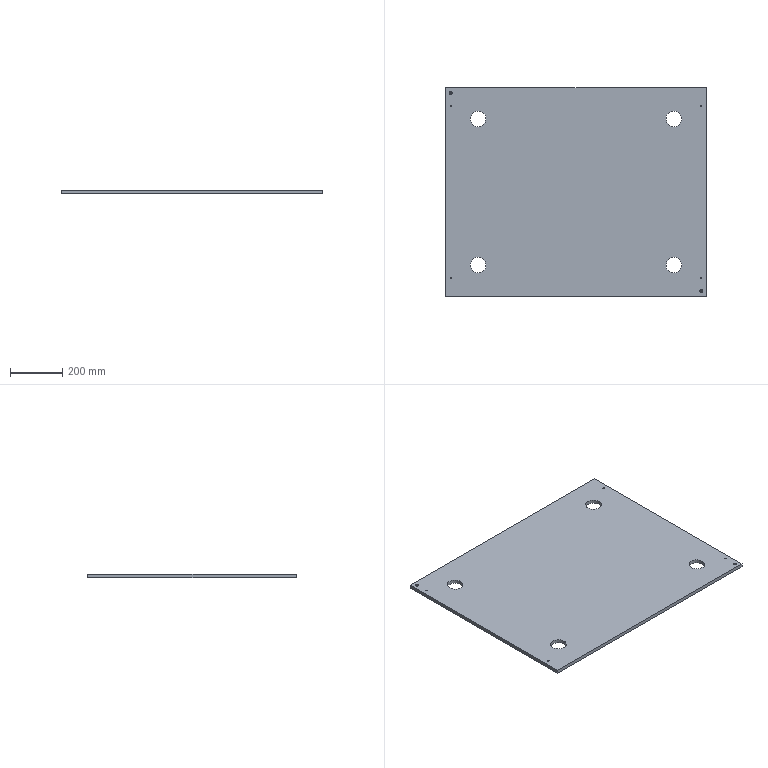Part | STEP file | Top plate | 1 solid | 40 faces | box 1000 x 800 x 14 mm | volume 11039590 mm3 | cylinder 24 | plane 12 | cone 4 | commonest cylinder face diameters 5.5 x12 60 x8 11 x4
STEP:
#1=CARTESIAN_POINT('',(-345.,-280.,0.));
#2=VERTEX_POINT('',#1);
#3=CARTESIAN_POINT('',(-405.,-280.,0.));
#4=VERTEX_POINT('',#3);
#5=CARTESIAN_POINT('',(-375.,-280.,0.));
#6=DIRECTION('',(0.,0.,-1.));
#7=DIRECTION('',(1.,0.,0.));
#8=AXIS2_PLACEMENT_3D('',#5,#6,#7);
#9=CIRCLE('',#8,30.);
#10=EDGE_CURVE('',#2,#4,#9,.T.);
#11=ORIENTED_EDGE('',*,*,#10,.T.);
#12=CARTESIAN_POINT('',(-405.,-280.,14.));
#13=VERTEX_POINT('',#12);
#14=CARTESIAN_POINT('',(-405.,-280.,-0.001));
#15=DIRECTION('',(0.,0.,1.));
#16=VECTOR('',#15,1000.);
#17=LINE('',#14,#16);
#18=EDGE_CURVE('',#4,#13,#17,.T.);
#19=ORIENTED_EDGE('',*,*,#18,.T.);
#20=CARTESIAN_POINT('',(-345.,-280.,14.));
#21=VERTEX_POINT('',#20);
#22=CARTESIAN_POINT('',(-375.,-280.,14.));
#23=DIRECTION('',(0.,0.,1.));
#24=DIRECTION('',(1.,0.,0.));
#25=AXIS2_PLACEMENT_3D('',#22,#23,#24);
#26=CIRCLE('',#25,30.);
#27=EDGE_CURVE('',#13,#21,#26,.T.);
#28=ORIENTED_EDGE('',*,*,#27,.T.);
#29=CARTESIAN_POINT('',(-345.,-280.,-0.001));
#30=DIRECTION('',(0.,0.,1.));
#31=VECTOR('',#30,1000.);
#32=LINE('',#29,#31);
#33=EDGE_CURVE('',#2,#21,#32,.T.);
#34=ORIENTED_EDGE('',*,*,#33,.F.);
#35=EDGE_LOOP('',(#11,#19,#28,#34));
#36=FACE_OUTER_BOUND('',#35,.T.);
#37=CARTESIAN_POINT('',(-375.,-280.,-0.001));
#38=DIRECTION('',(0.,0.,1.));
#39=DIRECTION('',(1.,0.,0.));
#40=AXIS2_PLACEMENT_3D('',#37,#38,#39);
#41=CYLINDRICAL_SURFACE('',#40,30.);
#42=ADVANCED_FACE('',(#36),#41,.F.);
#43=CARTESIAN_POINT('',(405.,-280.,0.));
#44=VERTEX_POINT('',#43);
#45=CARTESIAN_POINT('',(345.,-280.,0.));
#46=VERTEX_POINT('',#45);
#47=CARTESIAN_POINT('',(375.,-280.,0.));
#48=DIRECTION('',(0.,0.,-1.));
#49=DIRECTION('',(1.,0.,0.));
#50=AXIS2_PLACEMENT_3D('',#47,#48,#49);
#51=CIRCLE('',#50,30.);
#52=EDGE_CURVE('',#44,#46,#51,.T.);
#53=ORIENTED_EDGE('',*,*,#52,.T.);
#54=CARTESIAN_POINT('',(345.,-280.,14.));
#55=VERTEX_POINT('',#54);
#56=CARTESIAN_POINT('',(345.,-280.,-0.001));
#57=DIRECTION('',(0.,0.,1.));
#58=VECTOR('',#57,1000.);
#59=LINE('',#56,#58);
#60=EDGE_CURVE('',#46,#55,#59,.T.);
#61=ORIENTED_EDGE('',*,*,#60,.T.);
#62=CARTESIAN_POINT('',(405.,-280.,14.));
#63=VERTEX_POINT('',#62);
#64=CARTESIAN_POINT('',(375.,-280.,14.));
#65=DIRECTION('',(0.,0.,1.));
#66=DIRECTION('',(1.,0.,0.));
#67=AXIS2_PLACEMENT_3D('',#64,#65,#66);
#68=CIRCLE('',#67,30.);
#69=EDGE_CURVE('',#55,#63,#68,.T.);
#70=ORIENTED_EDGE('',*,*,#69,.T.);
#71=CARTESIAN_POINT('',(405.,-280.,-0.001));
#72=DIRECTION('',(0.,0.,1.));
#73=VECTOR('',#72,1000.);
#74=LINE('',#71,#73);
#75=EDGE_CURVE('',#44,#63,#74,.T.);
#76=ORIENTED_EDGE('',*,*,#75,.F.);
#77=EDGE_LOOP('',(#53,#61,#70,#76));
#78=FACE_OUTER_BOUND('',#77,.T.);
#79=CARTESIAN_POINT('',(375.,-280.,-0.001));
#80=DIRECTION('',(0.,0.,1.));
#81=DIRECTION('',(1.,0.,0.));
#82=AXIS2_PLACEMENT_3D('',#79,#80,#81);
#83=CYLINDRICAL_SURFACE('',#82,30.);
#84=ADVANCED_FACE('',(#78),#83,.F.);
#85=CARTESIAN_POINT('',(405.,280.,0.));
#86=VERTEX_POINT('',#85);
#87=CARTESIAN_POINT('',(345.,280.,0.));
#88=VERTEX_POINT('',#87);
#89=CARTESIAN_POINT('',(375.,280.,0.));
#90=DIRECTION('',(0.,0.,-1.));
#91=DIRECTION('',(1.,0.,0.));
#92=AXIS2_PLACEMENT_3D('',#89,#90,#91);
#93=CIRCLE('',#92,30.);
#94=EDGE_CURVE('',#86,#88,#93,.T.);
#95=ORIENTED_EDGE('',*,*,#94,.T.);
#96=CARTESIAN_POINT('',(345.,280.,14.));
#97=VERTEX_POINT('',#96);
#98=CARTESIAN_POINT('',(345.,280.,-0.001));
#99=DIRECTION('',(0.,0.,1.));
#100=VECTOR('',#99,1000.);
#101=LINE('',#98,#100);
#102=EDGE_CURVE('',#88,#97,#101,.T.);
#103=ORIENTED_EDGE('',*,*,#102,.T.);
#104=CARTESIAN_POINT('',(405.,280.,14.));
#105=VERTEX_POINT('',#104);
#106=CARTESIAN_POINT('',(375.,280.,14.));
#107=DIRECTION('',(0.,0.,1.));
#108=DIRECTION('',(1.,0.,0.));
#109=AXIS2_PLACEMENT_3D('',#106,#107,#108);
#110=CIRCLE('',#109,30.);
#111=EDGE_CURVE('',#97,#105,#110,.T.);
#112=ORIENTED_EDGE('',*,*,#111,.T.);
#113=CARTESIAN_POINT('',(405.,280.,-0.001));
#114=DIRECTION('',(0.,0.,1.));
#115=VECTOR('',#114,1000.);
#116=LINE('',#113,#115);
#117=EDGE_CURVE('',#86,#105,#116,.T.);
#118=ORIENTED_EDGE('',*,*,#117,.F.);
#119=EDGE_LOOP('',(#95,#103,#112,#118));
#120=FACE_OUTER_BOUND('',#119,.T.);
#121=CARTESIAN_POINT('',(375.,280.,-0.001));
#122=DIRECTION('',(0.,0.,1.));
#123=DIRECTION('',(1.,0.,0.));
#124=AXIS2_PLACEMENT_3D('',#121,#122,#123);
#125=CYLINDRICAL_SURFACE('',#124,30.);
#126=ADVANCED_FACE('',(#120),#125,.F.);
#127=CARTESIAN_POINT('',(-345.,280.,0.));
#128=VERTEX_POINT('',#127);
#129=CARTESIAN_POINT('',(-405.,280.,0.));
#130=VERTEX_POINT('',#129);
#131=CARTESIAN_POINT('',(-375.,280.,0.));
#132=DIRECTION('',(0.,0.,-1.));
#133=DIRECTION('',(1.,0.,0.));
#134=AXIS2_PLACEMENT_3D('',#131,#132,#133);
#135=CIRCLE('',#134,30.);
#136=EDGE_CURVE('',#128,#130,#135,.T.);
#137=ORIENTED_EDGE('',*,*,#136,.T.);
#138=CARTESIAN_POINT('',(-405.,280.,14.));
#139=VERTEX_POINT('',#138);
#140=CARTESIAN_POINT('',(-405.,280.,-0.001));
#141=DIRECTION('',(0.,0.,1.));
#142=VECTOR('',#141,1000.);
#143=LINE('',#140,#142);
#144=EDGE_CURVE('',#130,#139,#143,.T.);
#145=ORIENTED_EDGE('',*,*,#144,.T.);
#146=CARTESIAN_POINT('',(-345.,280.,14.));
#147=VERTEX_POINT('',#146);
#148=CARTESIAN_POINT('',(-375.,280.,14.));
#149=DIRECTION('',(0.,0.,1.));
#150=DIRECTION('',(1.,0.,0.));
#151=AXIS2_PLACEMENT_3D('',#148,#149,#150);
#152=CIRCLE('',#151,30.);
#153=EDGE_CURVE('',#139,#147,#152,.T.);
#154=ORIENTED_EDGE('',*,*,#153,.T.);
#155=CARTESIAN_POINT('',(-345.,280.,-0.001));
#156=DIRECTION('',(0.,0.,1.));
#157=VECTOR('',#156,1000.);
#158=LINE('',#155,#157);
#159=EDGE_CURVE('',#128,#147,#158,.T.);
#160=ORIENTED_EDGE('',*,*,#159,.F.);
#161=EDGE_LOOP('',(#137,#145,#154,#160));
#162=FACE_OUTER_BOUND('',#161,.T.);
#163=CARTESIAN_POINT('',(-375.,280.,-0.001));
#164=DIRECTION('',(0.,0.,1.));
#165=DIRECTION('',(1.,0.,0.));
#166=AXIS2_PLACEMENT_3D('',#163,#164,#165);
#167=CYLINDRICAL_SURFACE('',#166,30.);
#168=ADVANCED_FACE('',(#162),#167,.F.);
#169=CARTESIAN_POINT('',(-482.75,330.,0.));
#170=VERTEX_POINT('',#169);
#171=CARTESIAN_POINT('',(-477.25,330.,0.));
#172=VERTEX_POINT('',#171);
#173=CARTESIAN_POINT('',(-480.,330.,0.));
#174=DIRECTION('',(0.,0.,1.));
#175=DIRECTION('',(1.,0.,0.));
#176=AXIS2_PLACEMENT_3D('',#173,#174,#175);
#177=CIRCLE('',#176,2.75);
#178=EDGE_CURVE('',#170,#172,#177,.T.);
#179=ORIENTED_EDGE('',*,*,#178,.F.);
#180=CARTESIAN_POINT('',(-482.75,330.,14.));
#181=VERTEX_POINT('',#180);
#182=CARTESIAN_POINT('',(-482.75,330.,14.));
#183=DIRECTION('',(0.,0.,1.));
#184=VECTOR('',#183,1000.);
#185=LINE('',#182,#184);
#186=EDGE_CURVE('',#170,#181,#185,.T.);
#187=ORIENTED_EDGE('',*,*,#186,.T.);
#188=CARTESIAN_POINT('',(-477.25,330.,14.));
#189=VERTEX_POINT('',#188);
#190=CARTESIAN_POINT('',(-480.,330.,14.));
#191=DIRECTION('',(0.,0.,1.));
#192=DIRECTION('',(1.,0.,0.));
#193=AXIS2_PLACEMENT_3D('',#190,#191,#192);
#194=CIRCLE('',#193,2.75);
#195=EDGE_CURVE('',#181,#189,#194,.T.);
#196=ORIENTED_EDGE('',*,*,#195,.T.);
#197=CARTESIAN_POINT('',(-477.25,330.,14.));
#198=DIRECTION('',(0.,0.,1.));
#199=VECTOR('',#198,1000.);
#200=LINE('',#197,#199);
#201=EDGE_CURVE('',#172,#189,#200,.T.);
#202=ORIENTED_EDGE('',*,*,#201,.F.);
#203=EDGE_LOOP('',(#179,#187,#196,#202));
#204=FACE_OUTER_BOUND('',#203,.T.);
#205=CARTESIAN_POINT('',(-480.,330.,14.));
#206=DIRECTION('',(0.,0.,1.));
#207=DIRECTION('',(1.,0.,0.));
#208=AXIS2_PLACEMENT_3D('',#205,#206,#207);
#209=CYLINDRICAL_SURFACE('',#208,2.75);
#210=ADVANCED_FACE('',(#204),#209,.F.);
#211=CARTESIAN_POINT('',(477.25,330.,0.));
#212=VERTEX_POINT('',#211);
#213=CARTESIAN_POINT('',(482.75,330.,0.));
#214=VERTEX_POINT('',#213);
#215=CARTESIAN_POINT('',(480.,330.,0.));
#216=DIRECTION('',(0.,0.,1.));
#217=DIRECTION('',(1.,0.,0.));
#218=AXIS2_PLACEMENT_3D('',#215,#216,#217);
#219=CIRCLE('',#218,2.75);
#220=EDGE_CURVE('',#212,#214,#219,.T.);
#221=ORIENTED_EDGE('',*,*,#220,.F.);
#222=CARTESIAN_POINT('',(477.25,330.,14.));
#223=VERTEX_POINT('',#222);
#224=CARTESIAN_POINT('',(477.25,330.,14.));
#225=DIRECTION('',(0.,0.,1.));
#226=VECTOR('',#225,1000.);
#227=LINE('',#224,#226);
#228=EDGE_CURVE('',#212,#223,#227,.T.);
#229=ORIENTED_EDGE('',*,*,#228,.T.);
#230=CARTESIAN_POINT('',(482.75,330.,14.));
#231=VERTEX_POINT('',#230);
#232=CARTESIAN_POINT('',(480.,330.,14.));
#233=DIRECTION('',(0.,0.,1.));
#234=DIRECTION('',(1.,0.,0.));
#235=AXIS2_PLACEMENT_3D('',#232,#233,#234);
#236=CIRCLE('',#235,2.75);
#237=EDGE_CURVE('',#223,#231,#236,.T.);
#238=ORIENTED_EDGE('',*,*,#237,.T.);
#239=CARTESIAN_POINT('',(482.75,330.,14.));
#240=DIRECTION('',(0.,0.,1.));
#241=VECTOR('',#240,1000.);
#242=LINE('',#239,#241);
#243=EDGE_CURVE('',#214,#231,#242,.T.);
#244=ORIENTED_EDGE('',*,*,#243,.F.);
#245=EDGE_LOOP('',(#221,#229,#238,#244));
#246=FACE_OUTER_BOUND('',#245,.T.);
#247=CARTESIAN_POINT('',(480.,330.,14.));
#248=DIRECTION('',(0.,0.,1.));
#249=DIRECTION('',(1.,0.,0.));
#250=AXIS2_PLACEMENT_3D('',#247,#248,#249);
#251=CYLINDRICAL_SURFACE('',#250,2.75);
#252=ADVANCED_FACE('',(#246),#251,.F.);
#253=CARTESIAN_POINT('',(-482.75,-330.,0.));
#254=VERTEX_POINT('',#253);
#255=CARTESIAN_POINT('',(-477.25,-330.,0.));
#256=VERTEX_POINT('',#255);
#257=CARTESIAN_POINT('',(-480.,-330.,0.));
#258=DIRECTION('',(0.,0.,1.));
#259=DIRECTION('',(1.,0.,0.));
#260=AXIS2_PLACEMENT_3D('',#257,#258,#259);
#261=CIRCLE('',#260,2.75);
#262=EDGE_CURVE('',#254,#256,#261,.T.);
#263=ORIENTED_EDGE('',*,*,#262,.F.);
#264=CARTESIAN_POINT('',(-482.75,-330.,14.));
#265=VERTEX_POINT('',#264);
#266=CARTESIAN_POINT('',(-482.75,-330.,14.));
#267=DIRECTION('',(0.,0.,1.));
#268=VECTOR('',#267,1000.);
#269=LINE('',#266,#268);
#270=EDGE_CURVE('',#254,#265,#269,.T.);
#271=ORIENTED_EDGE('',*,*,#270,.T.);
#272=CARTESIAN_POINT('',(-477.25,-330.,14.));
#273=VERTEX_POINT('',#272);
#274=CARTESIAN_POINT('',(-480.,-330.,14.));
#275=DIRECTION('',(0.,0.,1.));
#276=DIRECTION('',(1.,0.,0.));
#277=AXIS2_PLACEMENT_3D('',#274,#275,#276);
#278=CIRCLE('',#277,2.75);
#279=EDGE_CURVE('',#265,#273,#278,.T.);
#280=ORIENTED_EDGE('',*,*,#279,.T.);
#281=CARTESIAN_POINT('',(-477.25,-330.,14.));
#282=DIRECTION('',(0.,0.,1.));
#283=VECTOR('',#282,1000.);
#284=LINE('',#281,#283);
#285=EDGE_CURVE('',#256,#273,#284,.T.);
#286=ORIENTED_EDGE('',*,*,#285,.F.);
#287=EDGE_LOOP('',(#263,#271,#280,#286));
#288=FACE_OUTER_BOUND('',#287,.T.);
#289=CARTESIAN_POINT('',(-480.,-330.,14.));
#290=DIRECTION('',(0.,0.,1.));
#291=DIRECTION('',(1.,0.,0.));
#292=AXIS2_PLACEMENT_3D('',#289,#290,#291);
#293=CYLINDRICAL_SURFACE('',#292,2.75);
#294=ADVANCED_FACE('',(#288),#293,.F.);
#295=CARTESIAN_POINT('',(477.25,-330.,0.));
#296=VERTEX_POINT('',#295);
#297=CARTESIAN_POINT('',(482.75,-330.,0.));
#298=VERTEX_POINT('',#297);
#299=CARTESIAN_POINT('',(480.,-330.,0.));
#300=DIRECTION('',(0.,0.,1.));
#301=DIRECTION('',(1.,0.,0.));
#302=AXIS2_PLACEMENT_3D('',#299,#300,#301);
#303=CIRCLE('',#302,2.75);
#304=EDGE_CURVE('',#296,#298,#303,.T.);
#305=ORIENTED_EDGE('',*,*,#304,.F.);
#306=CARTESIAN_POINT('',(477.25,-330.,14.));
#307=VERTEX_POINT('',#306);
#308=CARTESIAN_POINT('',(477.25,-330.,14.));
#309=DIRECTION('',(0.,0.,1.));
#310=VECTOR('',#309,1000.);
#311=LINE('',#308,#310);
#312=EDGE_CURVE('',#296,#307,#311,.T.);
#313=ORIENTED_EDGE('',*,*,#312,.T.);
#314=CARTESIAN_POINT('',(482.75,-330.,14.));
#315=VERTEX_POINT('',#314);
#316=CARTESIAN_POINT('',(480.,-330.,14.));
#317=DIRECTION('',(0.,0.,1.));
#318=DIRECTION('',(1.,0.,0.));
#319=AXIS2_PLACEMENT_3D('',#316,#317,#318);
#320=CIRCLE('',#319,2.75);
#321=EDGE_CURVE('',#307,#315,#320,.T.);
#322=ORIENTED_EDGE('',*,*,#321,.T.);
#323=CARTESIAN_POINT('',(482.75,-330.,14.));
#324=DIRECTION('',(0.,0.,1.));
#325=VECTOR('',#324,1000.);
#326=LINE('',#323,#325);
#327=EDGE_CURVE('',#298,#315,#326,.T.);
#328=ORIENTED_EDGE('',*,*,#327,.F.);
#329=EDGE_LOOP('',(#305,#313,#322,#328));
#330=FACE_OUTER_BOUND('',#329,.T.);
#331=CARTESIAN_POINT('',(480.,-330.,14.));
#332=DIRECTION('',(0.,0.,1.));
#333=DIRECTION('',(1.,0.,0.));
#334=AXIS2_PLACEMENT_3D('',#331,#332,#333);
#335=CYLINDRICAL_SURFACE('',#334,2.75);
#336=ADVANCED_FACE('',(#330),#335,.F.);
#337=CARTESIAN_POINT('',(-485.5,380.,13.975));
#338=VERTEX_POINT('',#337);
#339=CARTESIAN_POINT('',(-474.5,380.,13.975));
#340=VERTEX_POINT('',#339);
#341=CARTESIAN_POINT('',(-480.,380.,13.975));
#342=DIRECTION('',(0.,0.,1.));
#343=DIRECTION('',(1.,0.,0.));
#344=AXIS2_PLACEMENT_3D('',#341,#342,#343);
#345=CIRCLE('',#344,5.5);
#346=EDGE_CURVE('',#338,#340,#345,.T.);
#347=ORIENTED_EDGE('',*,*,#346,.F.);
#348=CARTESIAN_POINT('',(-485.525,380.,14.));
#349=VERTEX_POINT('',#348);
#350=CARTESIAN_POINT('',(-485.525,380.,14.));
#351=DIRECTION('',(-0.7071,0.,0.7071));
#352=VECTOR('',#351,1000.);
#353=LINE('',#350,#352);
#354=EDGE_CURVE('',#338,#349,#353,.T.);
#355=ORIENTED_EDGE('',*,*,#354,.T.);
#356=CARTESIAN_POINT('',(-474.475,380.,14.));
#357=VERTEX_POINT('',#356);
#358=CARTESIAN_POINT('',(-480.,380.,14.));
#359=DIRECTION('',(0.,0.,1.));
#360=DIRECTION('',(1.,0.,0.));
#361=AXIS2_PLACEMENT_3D('',#358,#359,#360);
#362=CIRCLE('',#361,5.525);
#363=EDGE_CURVE('',#349,#357,#362,.T.);
#364=ORIENTED_EDGE('',*,*,#363,.T.);
#365=CARTESIAN_POINT('',(-474.475,380.,14.));
#366=DIRECTION('',(0.7071,0.,0.7071));
#367=VECTOR('',#366,1000.);
#368=LINE('',#365,#367);
#369=EDGE_CURVE('',#340,#357,#368,.T.);
#370=ORIENTED_EDGE('',*,*,#369,.F.);
#371=EDGE_LOOP('',(#347,#355,#364,#370));
#372=FACE_OUTER_BOUND('',#371,.T.);
#373=CARTESIAN_POINT('',(-480.,380.,14.));
#374=DIRECTION('',(0.,0.,1.));
#375=DIRECTION('',(1.,0.,0.));
#376=AXIS2_PLACEMENT_3D('',#373,#374,#375);
#377=CONICAL_SURFACE('',#376,5.525,0.7854);
#378=ADVANCED_FACE('',(#372),#377,.F.);
#379=CARTESIAN_POINT('',(-485.5,380.,13.5));
#380=VERTEX_POINT('',#379);
#381=CARTESIAN_POINT('',(-474.5,380.,13.5));
#382=VERTEX_POINT('',#381);
#383=CARTESIAN_POINT('',(-480.,380.,13.5));
#384=DIRECTION('',(0.,0.,1.));
#385=DIRECTION('',(1.,0.,0.));
#386=AXIS2_PLACEMENT_3D('',#383,#384,#385);
#387=CIRCLE('',#386,5.5);
#388=EDGE_CURVE('',#380,#382,#387,.T.);
#389=ORIENTED_EDGE('',*,*,#388,.F.);
#390=CARTESIAN_POINT('',(-485.5,380.,14.));
#391=DIRECTION('',(0.,0.,1.));
#392=VECTOR('',#391,1000.);
#393=LINE('',#390,#392);
#394=EDGE_CURVE('',#380,#338,#393,.T.);
#395=ORIENTED_EDGE('',*,*,#394,.T.);
#396=ORIENTED_EDGE('',*,*,#346,.T.);
#397=CARTESIAN_POINT('',(-474.5,380.,14.));
#398=DIRECTION('',(0.,0.,1.));
#399=VECTOR('',#398,1000.);
#400=LINE('',#397,#399);
#401=EDGE_CURVE('',#382,#340,#400,.T.);
#402=ORIENTED_EDGE('',*,*,#401,.F.);
#403=EDGE_LOOP('',(#389,#395,#396,#402));
#404=FACE_OUTER_BOUND('',#403,.T.);
#405=CARTESIAN_POINT('',(-480.,380.,14.));
#406=DIRECTION('',(0.,0.,1.));
#407=DIRECTION('',(1.,0.,0.));
#408=AXIS2_PLACEMENT_3D('',#405,#406,#407);
#409=CYLINDRICAL_SURFACE('',#408,5.5);
#410=ADVANCED_FACE('',(#404),#409,.F.);
#411=CARTESIAN_POINT('',(-482.75,380.,0.));
#412=VERTEX_POINT('',#411);
#413=CARTESIAN_POINT('',(-477.25,380.,0.));
#414=VERTEX_POINT('',#413);
#415=CARTESIAN_POINT('',(-480.,380.,0.));
#416=DIRECTION('',(0.,0.,1.));
#417=DIRECTION('',(1.,0.,0.));
#418=AXIS2_PLACEMENT_3D('',#415,#416,#417);
#419=CIRCLE('',#418,2.75);
#420=EDGE_CURVE('',#412,#414,#419,.T.);
#421=ORIENTED_EDGE('',*,*,#420,.F.);
#422=CARTESIAN_POINT('',(-482.75,380.,13.5));
#423=VERTEX_POINT('',#422);
#424=CARTESIAN_POINT('',(-482.75,380.,14.));
#425=DIRECTION('',(0.,0.,1.));
#426=VECTOR('',#425,1000.);
#427=LINE('',#424,#426);
#428=EDGE_CURVE('',#412,#423,#427,.T.);
#429=ORIENTED_EDGE('',*,*,#428,.T.);
#430=CARTESIAN_POINT('',(-477.25,380.,13.5));
#431=VERTEX_POINT('',#430);
#432=CARTESIAN_POINT('',(-480.,380.,13.5));
#433=DIRECTION('',(0.,0.,1.));
#434=DIRECTION('',(1.,0.,0.));
#435=AXIS2_PLACEMENT_3D('',#432,#433,#434);
#436=CIRCLE('',#435,2.75);
#437=EDGE_CURVE('',#423,#431,#436,.T.);
#438=ORIENTED_EDGE('',*,*,#437,.T.);
#439=CARTESIAN_POINT('',(-477.25,380.,14.));
#440=DIRECTION('',(0.,0.,1.));
#441=VECTOR('',#440,1000.);
#442=LINE('',#439,#441);
#443=EDGE_CURVE('',#414,#431,#442,.T.);
#444=ORIENTED_EDGE('',*,*,#443,.F.);
#445=EDGE_LOOP('',(#421,#429,#438,#444));
#446=FACE_OUTER_BOUND('',#445,.T.);
#447=CARTESIAN_POINT('',(-480.,380.,14.));
#448=DIRECTION('',(0.,0.,1.));
#449=DIRECTION('',(1.,0.,0.));
#450=AXIS2_PLACEMENT_3D('',#447,#448,#449);
#451=CYLINDRICAL_SURFACE('',#450,2.75);
#452=ADVANCED_FACE('',(#446),#451,.F.);
#453=CARTESIAN_POINT('',(474.5,-380.,13.975));
#454=VERTEX_POINT('',#453);
#455=CARTESIAN_POINT('',(485.5,-380.,13.975));
#456=VERTEX_POINT('',#455);
#457=CARTESIAN_POINT('',(480.,-380.,13.975));
#458=DIRECTION('',(0.,0.,1.));
#459=DIRECTION('',(1.,0.,0.));
#460=AXIS2_PLACEMENT_3D('',#457,#458,#459);
#461=CIRCLE('',#460,5.5);
#462=EDGE_CURVE('',#454,#456,#461,.T.);
#463=ORIENTED_EDGE('',*,*,#462,.F.);
#464=CARTESIAN_POINT('',(474.475,-380.,14.));
#465=VERTEX_POINT('',#464);
#466=CARTESIAN_POINT('',(474.475,-380.,14.));
#467=DIRECTION('',(-0.7071,0.,0.7071));
#468=VECTOR('',#467,1000.);
#469=LINE('',#466,#468);
#470=EDGE_CURVE('',#454,#465,#469,.T.);
#471=ORIENTED_EDGE('',*,*,#470,.T.);
#472=CARTESIAN_POINT('',(485.525,-380.,14.));
#473=VERTEX_POINT('',#472);
#474=CARTESIAN_POINT('',(480.,-380.,14.));
#475=DIRECTION('',(0.,0.,1.));
#476=DIRECTION('',(1.,0.,0.));
#477=AXIS2_PLACEMENT_3D('',#474,#475,#476);
#478=CIRCLE('',#477,5.525);
#479=EDGE_CURVE('',#465,#473,#478,.T.);
#480=ORIENTED_EDGE('',*,*,#479,.T.);
#481=CARTESIAN_POINT('',(485.525,-380.,14.));
#482=DIRECTION('',(0.7071,0.,0.7071));
#483=VECTOR('',#482,1000.);
#484=LINE('',#481,#483);
#485=EDGE_CURVE('',#456,#473,#484,.T.);
#486=ORIENTED_EDGE('',*,*,#485,.F.);
#487=EDGE_LOOP('',(#463,#471,#480,#486));
#488=FACE_OUTER_BOUND('',#487,.T.);
#489=CARTESIAN_POINT('',(480.,-380.,14.));
#490=DIRECTION('',(0.,0.,1.));
#491=DIRECTION('',(1.,0.,0.));
#492=AXIS2_PLACEMENT_3D('',#489,#490,#491);
#493=CONICAL_SURFACE('',#492,5.525,0.7854);
#494=ADVANCED_FACE('',(#488),#493,.F.);
#495=CARTESIAN_POINT('',(474.5,-380.,13.5));
#496=VERTEX_POINT('',#495);
#497=CARTESIAN_POINT('',(485.5,-380.,13.5));
#498=VERTEX_POINT('',#497);
#499=CARTESIAN_POINT('',(480.,-380.,13.5));
#500=DIRECTION('',(0.,0.,1.));
#501=DIRECTION('',(1.,0.,0.));
#502=AXIS2_PLACEMENT_3D('',#499,#500,#501);
#503=CIRCLE('',#502,5.5);
#504=EDGE_CURVE('',#496,#498,#503,.T.);
#505=ORIENTED_EDGE('',*,*,#504,.F.);
#506=CARTESIAN_POINT('',(474.5,-380.,14.));
#507=DIRECTION('',(0.,0.,1.));
#508=VECTOR('',#507,1000.);
#509=LINE('',#506,#508);
#510=EDGE_CURVE('',#496,#454,#509,.T.);
#511=ORIENTED_EDGE('',*,*,#510,.T.);
#512=ORIENTED_EDGE('',*,*,#462,.T.);
#513=CARTESIAN_POINT('',(485.5,-380.,14.));
#514=DIRECTION('',(0.,0.,1.));
#515=VECTOR('',#514,1000.);
#516=LINE('',#513,#515);
#517=EDGE_CURVE('',#498,#456,#516,.T.);
#518=ORIENTED_EDGE('',*,*,#517,.F.);
#519=EDGE_LOOP('',(#505,#511,#512,#518));
#520=FACE_OUTER_BOUND('',#519,.T.);
#521=CARTESIAN_POINT('',(480.,-380.,14.));
#522=DIRECTION('',(0.,0.,1.));
#523=DIRECTION('',(1.,0.,0.));
#524=AXIS2_PLACEMENT_3D('',#521,#522,#523);
#525=CYLINDRICAL_SURFACE('',#524,5.5);
#526=ADVANCED_FACE('',(#520),#525,.F.);
#527=CARTESIAN_POINT('',(477.25,-380.,0.));
#528=VERTEX_POINT('',#527);
#529=CARTESIAN_POINT('',(482.75,-380.,0.));
#530=VERTEX_POINT('',#529);
#531=CARTESIAN_POINT('',(480.,-380.,0.));
#532=DIRECTION('',(0.,0.,1.));
#533=DIRECTION('',(1.,0.,0.));
#534=AXIS2_PLACEMENT_3D('',#531,#532,#533);
#535=CIRCLE('',#534,2.75);
#536=EDGE_CURVE('',#528,#530,#535,.T.);
#537=ORIENTED_EDGE('',*,*,#536,.F.);
#538=CARTESIAN_POINT('',(477.25,-380.,13.5));
#539=VERTEX_POINT('',#538);
#540=CARTESIAN_POINT('',(477.25,-380.,14.));
#541=DIRECTION('',(0.,0.,1.));
#542=VECTOR('',#541,1000.);
#543=LINE('',#540,#542);
#544=EDGE_CURVE('',#528,#539,#543,.T.);
#545=ORIENTED_EDGE('',*,*,#544,.T.);
#546=CARTESIAN_POINT('',(482.75,-380.,13.5));
#547=VERTEX_POINT('',#546);
#548=CARTESIAN_POINT('',(480.,-380.,13.5));
#549=DIRECTION('',(0.,0.,1.));
#550=DIRECTION('',(1.,0.,0.));
#551=AXIS2_PLACEMENT_3D('',#548,#549,#550);
#552=CIRCLE('',#551,2.75);
#553=EDGE_CURVE('',#539,#547,#552,.T.);
#554=ORIENTED_EDGE('',*,*,#553,.T.);
#555=CARTESIAN_POINT('',(482.75,-380.,14.));
#556=DIRECTION('',(0.,0.,1.));
#557=VECTOR('',#556,1000.);
#558=LINE('',#555,#557);
#559=EDGE_CURVE('',#530,#547,#558,.T.);
#560=ORIENTED_EDGE('',*,*,#559,.F.);
#561=EDGE_LOOP('',(#537,#545,#554,#560));
#562=FACE_OUTER_BOUND('',#561,.T.);
#563=CARTESIAN_POINT('',(480.,-380.,14.));
#564=DIRECTION('',(0.,0.,1.));
#565=DIRECTION('',(1.,0.,0.));
#566=AXIS2_PLACEMENT_3D('',#563,#564,#565);
#567=CYLINDRICAL_SURFACE('',#566,2.75);
#568=ADVANCED_FACE('',(#562),#567,.F.);
#569=CARTESIAN_POINT('',(500.,-399.5,14.));
#570=VERTEX_POINT('',#569);
#571=CARTESIAN_POINT('',(500.,399.5,14.));
#572=VERTEX_POINT('',#571);
#573=CARTESIAN_POINT('',(500.,-400.,14.));
#574=DIRECTION('',(0.,1.,0.));
#575=VECTOR('',#574,1000.);
#576=LINE('',#573,#575);
#577=EDGE_CURVE('',#570,#572,#576,.T.);
#578=ORIENTED_EDGE('',*,*,#577,.F.);
#579=CARTESIAN_POINT('',(500.,-399.5,0.));
#580=VERTEX_POINT('',#579);
#581=CARTESIAN_POINT('',(500.,-399.5,14.));
#582=DIRECTION('',(0.,0.,-1.));
#583=VECTOR('',#582,1000.);
#584=LINE('',#581,#583);
#585=EDGE_CURVE('',#570,#580,#584,.T.);
#586=ORIENTED_EDGE('',*,*,#585,.T.);
#587=CARTESIAN_POINT('',(500.,399.5,0.));
#588=VERTEX_POINT('',#587);
#589=CARTESIAN_POINT('',(500.,-400.,0.));
#590=DIRECTION('',(0.,1.,0.));
#591=VECTOR('',#590,1000.);
#592=LINE('',#589,#591);
#593=EDGE_CURVE('',#580,#588,#592,.T.);
#594=ORIENTED_EDGE('',*,*,#593,.T.);
#595=CARTESIAN_POINT('',(500.,399.5,14.));
#596=DIRECTION('',(0.,0.,1.));
#597=VECTOR('',#596,1000.);
#598=LINE('',#595,#597);
#599=EDGE_CURVE('',#588,#572,#598,.T.);
#600=ORIENTED_EDGE('',*,*,#599,.T.);
#601=EDGE_LOOP('',(#578,#586,#594,#600));
#602=FACE_OUTER_BOUND('',#601,.T.);
#603=CARTESIAN_POINT('',(500.,-400.,14.));
#604=DIRECTION('',(-1.,0.,0.));
#605=DIRECTION('',(0.,0.,1.));
#606=AXIS2_PLACEMENT_3D('',#603,#604,#605);
#607=PLANE('',#606);
#608=ADVANCED_FACE('',(#602),#607,.F.);
#609=CARTESIAN_POINT('',(499.5,400.,0.));
#610=VERTEX_POINT('',#609);
#611=CARTESIAN_POINT('',(-499.5,400.,0.));
#612=VERTEX_POINT('',#611);
#613=CARTESIAN_POINT('',(500.,400.,0.));
#614=DIRECTION('',(-1.,0.,0.));
#615=VECTOR('',#614,1000.);
#616=LINE('',#613,#615);
#617=EDGE_CURVE('',#610,#612,#616,.T.);
#618=ORIENTED_EDGE('',*,*,#617,.T.);
#619=CARTESIAN_POINT('',(-499.5,400.,14.));
#620=VERTEX_POINT('',#619);
#621=CARTESIAN_POINT('',(-499.5,400.,14.));
#622=DIRECTION('',(0.,0.,1.));
#623=VECTOR('',#622,1000.);
#624=LINE('',#621,#623);
#625=EDGE_CURVE('',#612,#620,#624,.T.);
#626=ORIENTED_EDGE('',*,*,#625,.T.);
#627=CARTESIAN_POINT('',(499.5,400.,14.));
#628=VERTEX_POINT('',#627);
#629=CARTESIAN_POINT('',(500.,400.,14.));
#630=DIRECTION('',(-1.,0.,0.));
#631=VECTOR('',#630,1000.);
#632=LINE('',#629,#631);
#633=EDGE_CURVE('',#628,#620,#632,.T.);
#634=ORIENTED_EDGE('',*,*,#633,.F.);
#635=CARTESIAN_POINT('',(499.5,400.,14.));
#636=DIRECTION('',(0.,0.,-1.));
#637=VECTOR('',#636,1000.);
#638=LINE('',#635,#637);
#639=EDGE_CURVE('',#628,#610,#638,.T.);
#640=ORIENTED_EDGE('',*,*,#639,.T.);
#641=EDGE_LOOP('',(#618,#626,#634,#640));
#642=FACE_OUTER_BOUND('',#641,.T.);
#643=CARTESIAN_POINT('',(500.,400.,14.));
#644=DIRECTION('',(0.,-1.,0.));
#645=DIRECTION('',(1.,0.,0.));
#646=AXIS2_PLACEMENT_3D('',#643,#644,#645);
#647=PLANE('',#646);
#648=ADVANCED_FACE('',(#642),#647,.F.);
#649=CARTESIAN_POINT('',(-500.,399.5,0.));
#650=VERTEX_POINT('',#649);
#651=CARTESIAN_POINT('',(-500.,-399.5,0.));
#652=VERTEX_POINT('',#651);
#653=CARTESIAN_POINT('',(-500.,-400.,0.));
#654=DIRECTION('',(0.,-1.,0.));
#655=VECTOR('',#654,1000.);
#656=LINE('',#653,#655);
#657=EDGE_CURVE('',#650,#652,#656,.T.);
#658=ORIENTED_EDGE('',*,*,#657,.T.);
#659=CARTESIAN_POINT('',(-500.,-399.5,14.));
#660=VERTEX_POINT('',#659);
#661=CARTESIAN_POINT('',(-500.,-399.5,14.));
#662=DIRECTION('',(0.,0.,1.));
#663=VECTOR('',#662,1000.);
#664=LINE('',#661,#663);
#665=EDGE_CURVE('',#652,#660,#664,.T.);
#666=ORIENTED_EDGE('',*,*,#665,.T.);
#667=CARTESIAN_POINT('',(-500.,399.5,14.));
#668=VERTEX_POINT('',#667);
#669=CARTESIAN_POINT('',(-500.,-400.,14.));
#670=DIRECTION('',(0.,-1.,0.));
#671=VECTOR('',#670,1000.);
#672=LINE('',#669,#671);
#673=EDGE_CURVE('',#668,#660,#672,.T.);
#674=ORIENTED_EDGE('',*,*,#673,.F.);
#675=CARTESIAN_POINT('',(-500.,399.5,14.));
#676=DIRECTION('',(0.,0.,-1.));
#677=VECTOR('',#676,1000.);
#678=LINE('',#675,#677);
#679=EDGE_CURVE('',#668,#650,#678,.T.);
#680=ORIENTED_EDGE('',*,*,#679,.T.);
#681=EDGE_LOOP('',(#658,#666,#674,#680));
#682=FACE_OUTER_BOUND('',#681,.T.);
#683=CARTESIAN_POINT('',(-500.,-400.,14.));
#684=DIRECTION('',(1.,0.,0.));
#685=DIRECTION('',(0.,0.,-1.));
#686=AXIS2_PLACEMENT_3D('',#683,#684,#685);
#687=PLANE('',#686);
#688=ADVANCED_FACE('',(#682),#687,.F.);
#689=CARTESIAN_POINT('',(-499.5,-400.,0.));
#690=VERTEX_POINT('',#689);
#691=CARTESIAN_POINT('',(499.5,-400.,0.));
#692=VERTEX_POINT('',#691);
#693=CARTESIAN_POINT('',(500.,-400.,0.));
#694=DIRECTION('',(1.,0.,0.));
#695=VECTOR('',#694,1000.);
#696=LINE('',#693,#695);
#697=EDGE_CURVE('',#690,#692,#696,.T.);
#698=ORIENTED_EDGE('',*,*,#697,.T.);
#699=CARTESIAN_POINT('',(499.5,-400.,14.));
#700=VERTEX_POINT('',#699);
#701=CARTESIAN_POINT('',(499.5,-400.,14.));
#702=DIRECTION('',(0.,0.,1.));
#703=VECTOR('',#702,1000.);
#704=LINE('',#701,#703);
#705=EDGE_CURVE('',#692,#700,#704,.T.);
#706=ORIENTED_EDGE('',*,*,#705,.T.);
#707=CARTESIAN_POINT('',(-499.5,-400.,14.));
#708=VERTEX_POINT('',#707);
#709=CARTESIAN_POINT('',(500.,-400.,14.));
#710=DIRECTION('',(1.,0.,0.));
#711=VECTOR('',#710,1000.);
#712=LINE('',#709,#711);
#713=EDGE_CURVE('',#708,#700,#712,.T.);
#714=ORIENTED_EDGE('',*,*,#713,.F.);
#715=CARTESIAN_POINT('',(-499.5,-400.,14.));
#716=DIRECTION('',(0.,0.,-1.));
#717=VECTOR('',#716,1000.);
#718=LINE('',#715,#717);
#719=EDGE_CURVE('',#708,#690,#718,.T.);
#720=ORIENTED_EDGE('',*,*,#719,.T.);
#721=EDGE_LOOP('',(#698,#706,#714,#720));
#722=FACE_OUTER_BOUND('',#721,.T.);
#723=CARTESIAN_POINT('',(500.,-400.,14.));
#724=DIRECTION('',(0.,1.,0.));
#725=DIRECTION('',(0.,0.,1.));
#726=AXIS2_PLACEMENT_3D('',#723,#724,#725);
#727=PLANE('',#726);
#728=ADVANCED_FACE('',(#722),#727,.F.);
#729=CARTESIAN_POINT('',(-375.,-280.,14.));
#730=DIRECTION('',(0.,0.,1.));
#731=DIRECTION('',(1.,0.,0.));
#732=AXIS2_PLACEMENT_3D('',#729,#730,#731);
#733=CIRCLE('',#732,30.);
#734=EDGE_CURVE('',#21,#13,#733,.T.);
#735=ORIENTED_EDGE('',*,*,#734,.F.);
#736=ORIENTED_EDGE('',*,*,#27,.F.);
#737=EDGE_LOOP('',(#735,#736));
#738=FACE_BOUND('',#737,.T.);
#739=CARTESIAN_POINT('',(375.,-280.,14.));
#740=DIRECTION('',(0.,0.,1.));
#741=DIRECTION('',(1.,0.,0.));
#742=AXIS2_PLACEMENT_3D('',#739,#740,#741);
#743=CIRCLE('',#742,30.);
#744=EDGE_CURVE('',#63,#55,#743,.T.);
#745=ORIENTED_EDGE('',*,*,#744,.F.);
#746=ORIENTED_EDGE('',*,*,#69,.F.);
#747=EDGE_LOOP('',(#745,#746));
#748=FACE_BOUND('',#747,.T.);
#749=CARTESIAN_POINT('',(375.,280.,14.));
#750=DIRECTION('',(0.,0.,1.));
#751=DIRECTION('',(1.,0.,0.));
#752=AXIS2_PLACEMENT_3D('',#749,#750,#751);
#753=CIRCLE('',#752,30.);
#754=EDGE_CURVE('',#105,#97,#753,.T.);
#755=ORIENTED_EDGE('',*,*,#754,.F.);
#756=ORIENTED_EDGE('',*,*,#111,.F.);
#757=EDGE_LOOP('',(#755,#756));
#758=FACE_BOUND('',#757,.T.);
#759=CARTESIAN_POINT('',(-375.,280.,14.));
#760=DIRECTION('',(0.,0.,1.));
#761=DIRECTION('',(1.,0.,0.));
#762=AXIS2_PLACEMENT_3D('',#759,#760,#761);
#763=CIRCLE('',#762,30.);
#764=EDGE_CURVE('',#147,#139,#763,.T.);
#765=ORIENTED_EDGE('',*,*,#764,.F.);
#766=ORIENTED_EDGE('',*,*,#153,.F.);
#767=EDGE_LOOP('',(#765,#766));
#768=FACE_BOUND('',#767,.T.);
#769=CARTESIAN_POINT('',(-480.,330.,14.));
#770=DIRECTION('',(0.,0.,1.));
#771=DIRECTION('',(1.,0.,0.));
#772=AXIS2_PLACEMENT_3D('',#769,#770,#771);
#773=CIRCLE('',#772,2.75);
#774=EDGE_CURVE('',#189,#181,#773,.T.);
#775=ORIENTED_EDGE('',*,*,#774,.F.);
#776=ORIENTED_EDGE('',*,*,#195,.F.);
#777=EDGE_LOOP('',(#775,#776));
#778=FACE_BOUND('',#777,.T.);
#779=CARTESIAN_POINT('',(480.,330.,14.));
#780=DIRECTION('',(0.,0.,1.));
#781=DIRECTION('',(1.,0.,0.));
#782=AXIS2_PLACEMENT_3D('',#779,#780,#781);
#783=CIRCLE('',#782,2.75);
#784=EDGE_CURVE('',#231,#223,#783,.T.);
#785=ORIENTED_EDGE('',*,*,#784,.F.);
#786=ORIENTED_EDGE('',*,*,#237,.F.);
#787=EDGE_LOOP('',(#785,#786));
#788=FACE_BOUND('',#787,.T.);
#789=CARTESIAN_POINT('',(-480.,-330.,14.));
#790=DIRECTION('',(0.,0.,1.));
#791=DIRECTION('',(1.,0.,0.));
#792=AXIS2_PLACEMENT_3D('',#789,#790,#791);
#793=CIRCLE('',#792,2.75);
#794=EDGE_CURVE('',#273,#265,#793,.T.);
#795=ORIENTED_EDGE('',*,*,#794,.F.);
#796=ORIENTED_EDGE('',*,*,#279,.F.);
#797=EDGE_LOOP('',(#795,#796));
#798=FACE_BOUND('',#797,.T.);
#799=CARTESIAN_POINT('',(480.,-330.,14.));
#800=DIRECTION('',(0.,0.,1.));
#801=DIRECTION('',(1.,0.,0.));
#802=AXIS2_PLACEMENT_3D('',#799,#800,#801);
#803=CIRCLE('',#802,2.75);
#804=EDGE_CURVE('',#315,#307,#803,.T.);
#805=ORIENTED_EDGE('',*,*,#804,.F.);
#806=ORIENTED_EDGE('',*,*,#321,.F.);
#807=EDGE_LOOP('',(#805,#806));
#808=FACE_BOUND('',#807,.T.);
#809=CARTESIAN_POINT('',(-480.,380.,14.));
#810=DIRECTION('',(0.,0.,1.));
#811=DIRECTION('',(1.,0.,0.));
#812=AXIS2_PLACEMENT_3D('',#809,#810,#811);
#813=CIRCLE('',#812,5.525);
#814=EDGE_CURVE('',#357,#349,#813,.T.);
#815=ORIENTED_EDGE('',*,*,#814,.F.);
#816=ORIENTED_EDGE('',*,*,#363,.F.);
#817=EDGE_LOOP('',(#815,#816));
#818=FACE_BOUND('',#817,.T.);
#819=CARTESIAN_POINT('',(480.,-380.,14.));
#820=DIRECTION('',(0.,0.,1.));
#821=DIRECTION('',(1.,0.,0.));
#822=AXIS2_PLACEMENT_3D('',#819,#820,#821);
#823=CIRCLE('',#822,5.525);
#824=EDGE_CURVE('',#473,#465,#823,.T.);
#825=ORIENTED_EDGE('',*,*,#824,.F.);
#826=ORIENTED_EDGE('',*,*,#479,.F.);
#827=EDGE_LOOP('',(#825,#826));
#828=FACE_BOUND('',#827,.T.);
#829=ORIENTED_EDGE('',*,*,#713,.T.);
#830=CARTESIAN_POINT('',(449.75,-449.75,14.));
#831=DIRECTION('',(0.7071,0.7071,0.));
#832=VECTOR('',#831,1000.);
#833=LINE('',#830,#832);
#834=EDGE_CURVE('',#700,#570,#833,.T.);
#835=ORIENTED_EDGE('',*,*,#834,.T.);
#836=ORIENTED_EDGE('',*,*,#577,.T.);
#837=CARTESIAN_POINT('',(449.75,449.75,14.));
#838=DIRECTION('',(-0.7071,0.7071,0.));
#839=VECTOR('',#838,1000.);
#840=LINE('',#837,#839);
#841=EDGE_CURVE('',#572,#628,#840,.T.);
#842=ORIENTED_EDGE('',*,*,#841,.T.);
#843=ORIENTED_EDGE('',*,*,#633,.T.);
#844=CARTESIAN_POINT('',(-449.75,449.75,14.));
#845=DIRECTION('',(-0.7071,-0.7071,0.));
#846=VECTOR('',#845,1000.);
#847=LINE('',#844,#846);
#848=EDGE_CURVE('',#620,#668,#847,.T.);
#849=ORIENTED_EDGE('',*,*,#848,.T.);
#850=ORIENTED_EDGE('',*,*,#673,.T.);
#851=CARTESIAN_POINT('',(-449.75,-449.75,14.));
#852=DIRECTION('',(0.7071,-0.7071,0.));
#853=VECTOR('',#852,1000.);
#854=LINE('',#851,#853);
#855=EDGE_CURVE('',#660,#708,#854,.T.);
#856=ORIENTED_EDGE('',*,*,#855,.T.);
#857=EDGE_LOOP('',(#829,#835,#836,#842,#843,#849,#850,#856));
#858=FACE_OUTER_BOUND('',#857,.T.);
#859=CARTESIAN_POINT('',(0.,0.,14.));
#860=DIRECTION('',(0.,0.,1.));
#861=DIRECTION('',(1.,0.,0.));
#862=AXIS2_PLACEMENT_3D('',#859,#860,#861);
#863=PLANE('',#862);
#864=ADVANCED_FACE('',(#738,#748,#758,#768,#778,#788,#798,#808,#818,#828,#858),#863,.T.);
#865=ORIENTED_EDGE('',*,*,#10,.F.);
#866=CARTESIAN_POINT('',(-375.,-280.,0.));
#867=DIRECTION('',(0.,0.,-1.));
#868=DIRECTION('',(1.,0.,0.));
#869=AXIS2_PLACEMENT_3D('',#866,#867,#868);
#870=CIRCLE('',#869,30.);
#871=EDGE_CURVE('',#4,#2,#870,.T.);
#872=ORIENTED_EDGE('',*,*,#871,.F.);
#873=EDGE_LOOP('',(#865,#872));
#874=FACE_BOUND('',#873,.T.);
#875=ORIENTED_EDGE('',*,*,#52,.F.);
#876=CARTESIAN_POINT('',(375.,-280.,0.));
#877=DIRECTION('',(0.,0.,-1.));
#878=DIRECTION('',(1.,0.,0.));
#879=AXIS2_PLACEMENT_3D('',#876,#877,#878);
#880=CIRCLE('',#879,30.);
#881=EDGE_CURVE('',#46,#44,#880,.T.);
#882=ORIENTED_EDGE('',*,*,#881,.F.);
#883=EDGE_LOOP('',(#875,#882));
#884=FACE_BOUND('',#883,.T.);
#885=ORIENTED_EDGE('',*,*,#94,.F.);
#886=CARTESIAN_POINT('',(375.,280.,0.));
#887=DIRECTION('',(0.,0.,-1.));
#888=DIRECTION('',(1.,0.,0.));
#889=AXIS2_PLACEMENT_3D('',#886,#887,#888);
#890=CIRCLE('',#889,30.);
#891=EDGE_CURVE('',#88,#86,#890,.T.);
#892=ORIENTED_EDGE('',*,*,#891,.F.);
#893=EDGE_LOOP('',(#885,#892));
#894=FACE_BOUND('',#893,.T.);
#895=ORIENTED_EDGE('',*,*,#136,.F.);
#896=CARTESIAN_POINT('',(-375.,280.,0.));
#897=DIRECTION('',(0.,0.,-1.));
#898=DIRECTION('',(1.,0.,0.));
#899=AXIS2_PLACEMENT_3D('',#896,#897,#898);
#900=CIRCLE('',#899,30.);
#901=EDGE_CURVE('',#130,#128,#900,.T.);
#902=ORIENTED_EDGE('',*,*,#901,.F.);
#903=EDGE_LOOP('',(#895,#902));
#904=FACE_BOUND('',#903,.T.);
#905=CARTESIAN_POINT('',(-480.,330.,0.));
#906=DIRECTION('',(0.,0.,1.));
#907=DIRECTION('',(1.,0.,0.));
#908=AXIS2_PLACEMENT_3D('',#905,#906,#907);
#909=CIRCLE('',#908,2.75);
#910=EDGE_CURVE('',#172,#170,#909,.T.);
#911=ORIENTED_EDGE('',*,*,#910,.T.);
#912=ORIENTED_EDGE('',*,*,#178,.T.);
#913=EDGE_LOOP('',(#911,#912));
#914=FACE_BOUND('',#913,.T.);
#915=CARTESIAN_POINT('',(480.,330.,0.));
#916=DIRECTION('',(0.,0.,1.));
#917=DIRECTION('',(1.,0.,0.));
#918=AXIS2_PLACEMENT_3D('',#915,#916,#917);
#919=CIRCLE('',#918,2.75);
#920=EDGE_CURVE('',#214,#212,#919,.T.);
#921=ORIENTED_EDGE('',*,*,#920,.T.);
#922=ORIENTED_EDGE('',*,*,#220,.T.);
#923=EDGE_LOOP('',(#921,#922));
#924=FACE_BOUND('',#923,.T.);
#925=CARTESIAN_POINT('',(-480.,-330.,0.));
#926=DIRECTION('',(0.,0.,1.));
#927=DIRECTION('',(1.,0.,0.));
#928=AXIS2_PLACEMENT_3D('',#925,#926,#927);
#929=CIRCLE('',#928,2.75);
#930=EDGE_CURVE('',#256,#254,#929,.T.);
#931=ORIENTED_EDGE('',*,*,#930,.T.);
#932=ORIENTED_EDGE('',*,*,#262,.T.);
#933=EDGE_LOOP('',(#931,#932));
#934=FACE_BOUND('',#933,.T.);
#935=CARTESIAN_POINT('',(480.,-330.,0.));
#936=DIRECTION('',(0.,0.,1.));
#937=DIRECTION('',(1.,0.,0.));
#938=AXIS2_PLACEMENT_3D('',#935,#936,#937);
#939=CIRCLE('',#938,2.75);
#940=EDGE_CURVE('',#298,#296,#939,.T.);
#941=ORIENTED_EDGE('',*,*,#940,.T.);
#942=ORIENTED_EDGE('',*,*,#304,.T.);
#943=EDGE_LOOP('',(#941,#942));
#944=FACE_BOUND('',#943,.T.);
#945=CARTESIAN_POINT('',(-480.,380.,0.));
#946=DIRECTION('',(0.,0.,1.));
#947=DIRECTION('',(1.,0.,0.));
#948=AXIS2_PLACEMENT_3D('',#945,#946,#947);
#949=CIRCLE('',#948,2.75);
#950=EDGE_CURVE('',#414,#412,#949,.T.);
#951=ORIENTED_EDGE('',*,*,#950,.T.);
#952=ORIENTED_EDGE('',*,*,#420,.T.);
#953=EDGE_LOOP('',(#951,#952));
#954=FACE_BOUND('',#953,.T.);
#955=CARTESIAN_POINT('',(480.,-380.,0.));
#956=DIRECTION('',(0.,0.,1.));
#957=DIRECTION('',(1.,0.,0.));
#958=AXIS2_PLACEMENT_3D('',#955,#956,#957);
#959=CIRCLE('',#958,2.75);
#960=EDGE_CURVE('',#530,#528,#959,.T.);
#961=ORIENTED_EDGE('',*,*,#960,.T.);
#962=ORIENTED_EDGE('',*,*,#536,.T.);
#963=EDGE_LOOP('',(#961,#962));
#964=FACE_BOUND('',#963,.T.);
#965=ORIENTED_EDGE('',*,*,#593,.F.);
#966=CARTESIAN_POINT('',(500.,-399.5,0.));
#967=DIRECTION('',(-0.7071,-0.7071,0.));
#968=VECTOR('',#967,1000.);
#969=LINE('',#966,#968);
#970=EDGE_CURVE('',#580,#692,#969,.T.);
#971=ORIENTED_EDGE('',*,*,#970,.T.);
#972=ORIENTED_EDGE('',*,*,#697,.F.);
#973=CARTESIAN_POINT('',(-499.5,-400.,0.));
#974=DIRECTION('',(-0.7071,0.7071,0.));
#975=VECTOR('',#974,1000.);
#976=LINE('',#973,#975);
#977=EDGE_CURVE('',#690,#652,#976,.T.);
#978=ORIENTED_EDGE('',*,*,#977,.T.);
#979=ORIENTED_EDGE('',*,*,#657,.F.);
#980=CARTESIAN_POINT('',(-500.,399.5,0.));
#981=DIRECTION('',(0.7071,0.7071,0.));
#982=VECTOR('',#981,1000.);
#983=LINE('',#980,#982);
#984=EDGE_CURVE('',#650,#612,#983,.T.);
#985=ORIENTED_EDGE('',*,*,#984,.T.);
#986=ORIENTED_EDGE('',*,*,#617,.F.);
#987=CARTESIAN_POINT('',(499.5,400.,0.));
#988=DIRECTION('',(0.7071,-0.7071,0.));
#989=VECTOR('',#988,1000.);
#990=LINE('',#987,#989);
#991=EDGE_CURVE('',#610,#588,#990,.T.);
#992=ORIENTED_EDGE('',*,*,#991,.T.);
#993=EDGE_LOOP('',(#965,#971,#972,#978,#979,#985,#986,#992));
#994=FACE_OUTER_BOUND('',#993,.T.);
#995=CARTESIAN_POINT('',(0.,0.,0.));
#996=DIRECTION('',(0.,0.,1.));
#997=DIRECTION('',(1.,0.,0.));
#998=AXIS2_PLACEMENT_3D('',#995,#996,#997);
#999=PLANE('',#998);
#1000=ADVANCED_FACE('',(#874,#884,#894,#904,#914,#924,#934,#944,#954,#964,#994),#999,.F.);
#1001=ORIENTED_EDGE('',*,*,#544,.F.);
#1002=ORIENTED_EDGE('',*,*,#960,.F.);
#1003=ORIENTED_EDGE('',*,*,#559,.T.);
#1004=CARTESIAN_POINT('',(480.,-380.,13.5));
#1005=DIRECTION('',(0.,0.,1.));
#1006=DIRECTION('',(1.,0.,0.));
#1007=AXIS2_PLACEMENT_3D('',#1004,#1005,#1006);
#1008=CIRCLE('',#1007,2.75);
#1009=EDGE_CURVE('',#547,#539,#1008,.T.);
#1010=ORIENTED_EDGE('',*,*,#1009,.T.);
#1011=EDGE_LOOP('',(#1001,#1002,#1003,#1010));
#1012=FACE_OUTER_BOUND('',#1011,.T.);
#1013=CARTESIAN_POINT('',(480.,-380.,14.));
#1014=DIRECTION('',(0.,0.,1.));
#1015=DIRECTION('',(1.,0.,0.));
#1016=AXIS2_PLACEMENT_3D('',#1013,#1014,#1015);
#1017=CYLINDRICAL_SURFACE('',#1016,2.75);
#1018=ADVANCED_FACE('',(#1012),#1017,.F.);
#1019=ORIENTED_EDGE('',*,*,#1009,.F.);
#1020=ORIENTED_EDGE('',*,*,#553,.F.);
#1021=EDGE_LOOP('',(#1019,#1020));
#1022=FACE_BOUND('',#1021,.T.);
#1023=CARTESIAN_POINT('',(480.,-380.,13.5));
#1024=DIRECTION('',(0.,0.,1.));
#1025=DIRECTION('',(1.,0.,0.));
#1026=AXIS2_PLACEMENT_3D('',#1023,#1024,#1025);
#1027=CIRCLE('',#1026,5.5);
#1028=EDGE_CURVE('',#498,#496,#1027,.T.);
#1029=ORIENTED_EDGE('',*,*,#1028,.T.);
#1030=ORIENTED_EDGE('',*,*,#504,.T.);
#1031=EDGE_LOOP('',(#1029,#1030));
#1032=FACE_OUTER_BOUND('',#1031,.T.);
#1033=CARTESIAN_POINT('',(485.5,-380.,13.5));
#1034=DIRECTION('',(0.,0.,-1.));
#1035=DIRECTION('',(-1.,0.,0.));
#1036=AXIS2_PLACEMENT_3D('',#1033,#1034,#1035);
#1037=PLANE('',#1036);
#1038=ADVANCED_FACE('',(#1022,#1032),#1037,.F.);
#1039=ORIENTED_EDGE('',*,*,#510,.F.);
#1040=ORIENTED_EDGE('',*,*,#1028,.F.);
#1041=ORIENTED_EDGE('',*,*,#517,.T.);
#1042=CARTESIAN_POINT('',(480.,-380.,13.975));
#1043=DIRECTION('',(0.,0.,1.));
#1044=DIRECTION('',(1.,0.,0.));
#1045=AXIS2_PLACEMENT_3D('',#1042,#1043,#1044);
#1046=CIRCLE('',#1045,5.5);
#1047=EDGE_CURVE('',#456,#454,#1046,.T.);
#1048=ORIENTED_EDGE('',*,*,#1047,.T.);
#1049=EDGE_LOOP('',(#1039,#1040,#1041,#1048));
#1050=FACE_OUTER_BOUND('',#1049,.T.);
#1051=CARTESIAN_POINT('',(480.,-380.,14.));
#1052=DIRECTION('',(0.,0.,1.));
#1053=DIRECTION('',(1.,0.,0.));
#1054=AXIS2_PLACEMENT_3D('',#1051,#1052,#1053);
#1055=CYLINDRICAL_SURFACE('',#1054,5.5);
#1056=ADVANCED_FACE('',(#1050),#1055,.F.);
#1057=ORIENTED_EDGE('',*,*,#470,.F.);
#1058=ORIENTED_EDGE('',*,*,#1047,.F.);
#1059=ORIENTED_EDGE('',*,*,#485,.T.);
#1060=ORIENTED_EDGE('',*,*,#824,.T.);
#1061=EDGE_LOOP('',(#1057,#1058,#1059,#1060));
#1062=FACE_OUTER_BOUND('',#1061,.T.);
#1063=CARTESIAN_POINT('',(480.,-380.,14.));
#1064=DIRECTION('',(0.,0.,1.));
#1065=DIRECTION('',(1.,0.,0.));
#1066=AXIS2_PLACEMENT_3D('',#1063,#1064,#1065);
#1067=CONICAL_SURFACE('',#1066,5.525,0.7854);
#1068=ADVANCED_FACE('',(#1062),#1067,.F.);
#1069=ORIENTED_EDGE('',*,*,#428,.F.);
#1070=ORIENTED_EDGE('',*,*,#950,.F.);
#1071=ORIENTED_EDGE('',*,*,#443,.T.);
#1072=CARTESIAN_POINT('',(-480.,380.,13.5));
#1073=DIRECTION('',(0.,0.,1.));
#1074=DIRECTION('',(1.,0.,0.));
#1075=AXIS2_PLACEMENT_3D('',#1072,#1073,#1074);
#1076=CIRCLE('',#1075,2.75);
#1077=EDGE_CURVE('',#431,#423,#1076,.T.);
#1078=ORIENTED_EDGE('',*,*,#1077,.T.);
#1079=EDGE_LOOP('',(#1069,#1070,#1071,#1078));
#1080=FACE_OUTER_BOUND('',#1079,.T.);
#1081=CARTESIAN_POINT('',(-480.,380.,14.));
#1082=DIRECTION('',(0.,0.,1.));
#1083=DIRECTION('',(1.,0.,0.));
#1084=AXIS2_PLACEMENT_3D('',#1081,#1082,#1083);
#1085=CYLINDRICAL_SURFACE('',#1084,2.75);
#1086=ADVANCED_FACE('',(#1080),#1085,.F.);
#1087=ORIENTED_EDGE('',*,*,#1077,.F.);
#1088=ORIENTED_EDGE('',*,*,#437,.F.);
#1089=EDGE_LOOP('',(#1087,#1088));
#1090=FACE_BOUND('',#1089,.T.);
#1091=CARTESIAN_POINT('',(-480.,380.,13.5));
#1092=DIRECTION('',(0.,0.,1.));
#1093=DIRECTION('',(1.,0.,0.));
#1094=AXIS2_PLACEMENT_3D('',#1091,#1092,#1093);
#1095=CIRCLE('',#1094,5.5);
#1096=EDGE_CURVE('',#382,#380,#1095,.T.);
#1097=ORIENTED_EDGE('',*,*,#1096,.T.);
#1098=ORIENTED_EDGE('',*,*,#388,.T.);
#1099=EDGE_LOOP('',(#1097,#1098));
#1100=FACE_OUTER_BOUND('',#1099,.T.);
#1101=CARTESIAN_POINT('',(-474.5,380.,13.5));
#1102=DIRECTION('',(0.,0.,-1.));
#1103=DIRECTION('',(-1.,0.,0.));
#1104=AXIS2_PLACEMENT_3D('',#1101,#1102,#1103);
#1105=PLANE('',#1104);
#1106=ADVANCED_FACE('',(#1090,#1100),#1105,.F.);
#1107=ORIENTED_EDGE('',*,*,#394,.F.);
#1108=ORIENTED_EDGE('',*,*,#1096,.F.);
#1109=ORIENTED_EDGE('',*,*,#401,.T.);
#1110=CARTESIAN_POINT('',(-480.,380.,13.975));
#1111=DIRECTION('',(0.,0.,1.));
#1112=DIRECTION('',(1.,0.,0.));
#1113=AXIS2_PLACEMENT_3D('',#1110,#1111,#1112);
#1114=CIRCLE('',#1113,5.5);
#1115=EDGE_CURVE('',#340,#338,#1114,.T.);
#1116=ORIENTED_EDGE('',*,*,#1115,.T.);
#1117=EDGE_LOOP('',(#1107,#1108,#1109,#1116));
#1118=FACE_OUTER_BOUND('',#1117,.T.);
#1119=CARTESIAN_POINT('',(-480.,380.,14.));
#1120=DIRECTION('',(0.,0.,1.));
#1121=DIRECTION('',(1.,0.,0.));
#1122=AXIS2_PLACEMENT_3D('',#1119,#1120,#1121);
#1123=CYLINDRICAL_SURFACE('',#1122,5.5);
#1124=ADVANCED_FACE('',(#1118),#1123,.F.);
#1125=ORIENTED_EDGE('',*,*,#354,.F.);
#1126=ORIENTED_EDGE('',*,*,#1115,.F.);
#1127=ORIENTED_EDGE('',*,*,#369,.T.);
#1128=ORIENTED_EDGE('',*,*,#814,.T.);
#1129=EDGE_LOOP('',(#1125,#1126,#1127,#1128));
#1130=FACE_OUTER_BOUND('',#1129,.T.);
#1131=CARTESIAN_POINT('',(-480.,380.,14.));
#1132=DIRECTION('',(0.,0.,1.));
#1133=DIRECTION('',(1.,0.,0.));
#1134=AXIS2_PLACEMENT_3D('',#1131,#1132,#1133);
#1135=CONICAL_SURFACE('',#1134,5.525,0.7854);
#1136=ADVANCED_FACE('',(#1130),#1135,.F.);
#1137=ORIENTED_EDGE('',*,*,#834,.F.);
#1138=ORIENTED_EDGE('',*,*,#705,.F.);
#1139=ORIENTED_EDGE('',*,*,#970,.F.);
#1140=ORIENTED_EDGE('',*,*,#585,.F.);
#1141=EDGE_LOOP('',(#1137,#1138,#1139,#1140));
#1142=FACE_OUTER_BOUND('',#1141,.T.);
#1143=CARTESIAN_POINT('',(500.,-399.5,14.));
#1144=DIRECTION('',(-0.7071,0.7071,0.));
#1145=DIRECTION('',(0.,0.,-1.));
#1146=AXIS2_PLACEMENT_3D('',#1143,#1144,#1145);
#1147=PLANE('',#1146);
#1148=ADVANCED_FACE('',(#1142),#1147,.F.);
#1149=ORIENTED_EDGE('',*,*,#855,.F.);
#1150=ORIENTED_EDGE('',*,*,#665,.F.);
#1151=ORIENTED_EDGE('',*,*,#977,.F.);
#1152=ORIENTED_EDGE('',*,*,#719,.F.);
#1153=EDGE_LOOP('',(#1149,#1150,#1151,#1152));
#1154=FACE_OUTER_BOUND('',#1153,.T.);
#1155=CARTESIAN_POINT('',(-499.5,-400.,14.));
#1156=DIRECTION('',(0.7071,0.7071,0.));
#1157=DIRECTION('',(0.,0.,-1.));
#1158=AXIS2_PLACEMENT_3D('',#1155,#1156,#1157);
#1159=PLANE('',#1158);
#1160=ADVANCED_FACE('',(#1154),#1159,.F.);
#1161=ORIENTED_EDGE('',*,*,#848,.F.);
#1162=ORIENTED_EDGE('',*,*,#625,.F.);
#1163=ORIENTED_EDGE('',*,*,#984,.F.);
#1164=ORIENTED_EDGE('',*,*,#679,.F.);
#1165=EDGE_LOOP('',(#1161,#1162,#1163,#1164));
#1166=FACE_OUTER_BOUND('',#1165,.T.);
#1167=CARTESIAN_POINT('',(-500.,399.5,14.));
#1168=DIRECTION('',(0.7071,-0.7071,0.));
#1169=DIRECTION('',(0.,0.,-1.));
#1170=AXIS2_PLACEMENT_3D('',#1167,#1168,#1169);
#1171=PLANE('',#1170);
#1172=ADVANCED_FACE('',(#1166),#1171,.F.);
#1173=ORIENTED_EDGE('',*,*,#841,.F.);
#1174=ORIENTED_EDGE('',*,*,#599,.F.);
#1175=ORIENTED_EDGE('',*,*,#991,.F.);
#1176=ORIENTED_EDGE('',*,*,#639,.F.);
#1177=EDGE_LOOP('',(#1173,#1174,#1175,#1176));
#1178=FACE_OUTER_BOUND('',#1177,.T.);
#1179=CARTESIAN_POINT('',(499.5,400.,14.));
#1180=DIRECTION('',(-0.7071,-0.7071,0.));
#1181=DIRECTION('',(0.,0.,-1.));
#1182=AXIS2_PLACEMENT_3D('',#1179,#1180,#1181);
#1183=PLANE('',#1182);
#1184=ADVANCED_FACE('',(#1178),#1183,.F.);
#1185=ORIENTED_EDGE('',*,*,#312,.F.);
#1186=ORIENTED_EDGE('',*,*,#940,.F.);
#1187=ORIENTED_EDGE('',*,*,#327,.T.);
#1188=ORIENTED_EDGE('',*,*,#804,.T.);
#1189=EDGE_LOOP('',(#1185,#1186,#1187,#1188));
#1190=FACE_OUTER_BOUND('',#1189,.T.);
#1191=CARTESIAN_POINT('',(480.,-330.,14.));
#1192=DIRECTION('',(0.,0.,1.));
#1193=DIRECTION('',(1.,0.,0.));
#1194=AXIS2_PLACEMENT_3D('',#1191,#1192,#1193);
#1195=CYLINDRICAL_SURFACE('',#1194,2.75);
#1196=ADVANCED_FACE('',(#1190),#1195,.F.);
#1197=ORIENTED_EDGE('',*,*,#270,.F.);
#1198=ORIENTED_EDGE('',*,*,#930,.F.);
#1199=ORIENTED_EDGE('',*,*,#285,.T.);
#1200=ORIENTED_EDGE('',*,*,#794,.T.);
#1201=EDGE_LOOP('',(#1197,#1198,#1199,#1200));
#1202=FACE_OUTER_BOUND('',#1201,.T.);
#1203=CARTESIAN_POINT('',(-480.,-330.,14.));
#1204=DIRECTION('',(0.,0.,1.));
#1205=DIRECTION('',(1.,0.,0.));
#1206=AXIS2_PLACEMENT_3D('',#1203,#1204,#1205);
#1207=CYLINDRICAL_SURFACE('',#1206,2.75);
#1208=ADVANCED_FACE('',(#1202),#1207,.F.);
#1209=ORIENTED_EDGE('',*,*,#228,.F.);
#1210=ORIENTED_EDGE('',*,*,#920,.F.);
#1211=ORIENTED_EDGE('',*,*,#243,.T.);
#1212=ORIENTED_EDGE('',*,*,#784,.T.);
#1213=EDGE_LOOP('',(#1209,#1210,#1211,#1212));
#1214=FACE_OUTER_BOUND('',#1213,.T.);
#1215=CARTESIAN_POINT('',(480.,330.,14.));
#1216=DIRECTION('',(0.,0.,1.));
#1217=DIRECTION('',(1.,0.,0.));
#1218=AXIS2_PLACEMENT_3D('',#1215,#1216,#1217);
#1219=CYLINDRICAL_SURFACE('',#1218,2.75);
#1220=ADVANCED_FACE('',(#1214),#1219,.F.);
#1221=ORIENTED_EDGE('',*,*,#186,.F.);
#1222=ORIENTED_EDGE('',*,*,#910,.F.);
#1223=ORIENTED_EDGE('',*,*,#201,.T.);
#1224=ORIENTED_EDGE('',*,*,#774,.T.);
#1225=EDGE_LOOP('',(#1221,#1222,#1223,#1224));
#1226=FACE_OUTER_BOUND('',#1225,.T.);
#1227=CARTESIAN_POINT('',(-480.,330.,14.));
#1228=DIRECTION('',(0.,0.,1.));
#1229=DIRECTION('',(1.,0.,0.));
#1230=AXIS2_PLACEMENT_3D('',#1227,#1228,#1229);
#1231=CYLINDRICAL_SURFACE('',#1230,2.75);
#1232=ADVANCED_FACE('',(#1226),#1231,.F.);
#1233=ORIENTED_EDGE('',*,*,#144,.F.);
#1234=ORIENTED_EDGE('',*,*,#901,.T.);
#1235=ORIENTED_EDGE('',*,*,#159,.T.);
#1236=ORIENTED_EDGE('',*,*,#764,.T.);
#1237=EDGE_LOOP('',(#1233,#1234,#1235,#1236));
#1238=FACE_OUTER_BOUND('',#1237,.T.);
#1239=CARTESIAN_POINT('',(-375.,280.,-0.001));
#1240=DIRECTION('',(0.,0.,1.));
#1241=DIRECTION('',(1.,0.,0.));
#1242=AXIS2_PLACEMENT_3D('',#1239,#1240,#1241);
#1243=CYLINDRICAL_SURFACE('',#1242,30.);
#1244=ADVANCED_FACE('',(#1238),#1243,.F.);
#1245=ORIENTED_EDGE('',*,*,#102,.F.);
#1246=ORIENTED_EDGE('',*,*,#891,.T.);
#1247=ORIENTED_EDGE('',*,*,#117,.T.);
#1248=ORIENTED_EDGE('',*,*,#754,.T.);
#1249=EDGE_LOOP('',(#1245,#1246,#1247,#1248));
#1250=FACE_OUTER_BOUND('',#1249,.T.);
#1251=CARTESIAN_POINT('',(375.,280.,-0.001));
#1252=DIRECTION('',(0.,0.,1.));
#1253=DIRECTION('',(1.,0.,0.));
#1254=AXIS2_PLACEMENT_3D('',#1251,#1252,#1253);
#1255=CYLINDRICAL_SURFACE('',#1254,30.);
#1256=ADVANCED_FACE('',(#1250),#1255,.F.);
#1257=ORIENTED_EDGE('',*,*,#60,.F.);
#1258=ORIENTED_EDGE('',*,*,#881,.T.);
#1259=ORIENTED_EDGE('',*,*,#75,.T.);
#1260=ORIENTED_EDGE('',*,*,#744,.T.);
#1261=EDGE_LOOP('',(#1257,#1258,#1259,#1260));
#1262=FACE_OUTER_BOUND('',#1261,.T.);
#1263=CARTESIAN_POINT('',(375.,-280.,-0.001));
#1264=DIRECTION('',(0.,0.,1.));
#1265=DIRECTION('',(1.,0.,0.));
#1266=AXIS2_PLACEMENT_3D('',#1263,#1264,#1265);
#1267=CYLINDRICAL_SURFACE('',#1266,30.);
#1268=ADVANCED_FACE('',(#1262),#1267,.F.);
#1269=ORIENTED_EDGE('',*,*,#18,.F.);
#1270=ORIENTED_EDGE('',*,*,#871,.T.);
#1271=ORIENTED_EDGE('',*,*,#33,.T.);
#1272=ORIENTED_EDGE('',*,*,#734,.T.);
#1273=EDGE_LOOP('',(#1269,#1270,#1271,#1272));
#1274=FACE_OUTER_BOUND('',#1273,.T.);
#1275=CARTESIAN_POINT('',(-375.,-280.,-0.001));
#1276=DIRECTION('',(0.,0.,1.));
#1277=DIRECTION('',(1.,0.,0.));
#1278=AXIS2_PLACEMENT_3D('',#1275,#1276,#1277);
#1279=CYLINDRICAL_SURFACE('',#1278,30.);
#1280=ADVANCED_FACE('',(#1274),#1279,.F.);
#1281=CLOSED_SHELL('',(#42,#84,#126,#168,#210,#252,#294,#336,#378,#410,#452,#494,#526,#568,#608,#648,#688,#728,#864,#1000,#1018,#1038,#1056,#1068,#1086,#1106,#1124,#1136,#1148,#1160,#1172,#1184,#1196,#1208,#1220,#1232,#1244,#1256,#1268,#1280));
#1282=MANIFOLD_SOLID_BREP('',#1281);
#1283=CARTESIAN_POINT('',(0.,0.,0.));
#1284=DIRECTION('',(0.,0.,1.));
#1285=DIRECTION('',(1.,0.,0.));
#1286=AXIS2_PLACEMENT_3D('',#1283,#1284,#1285);
#1287=(LENGTH_UNIT()NAMED_UNIT(*)SI_UNIT(.MILLI.,.METRE.));
#1288=UNCERTAINTY_MEASURE_WITH_UNIT(LENGTH_MEASURE(0.00001),#1287,'','');
#1289=(NAMED_UNIT(*)PLANE_ANGLE_UNIT()SI_UNIT($,.RADIAN.));
#1290=(NAMED_UNIT(*)SI_UNIT($,.STERADIAN.)SOLID_ANGLE_UNIT());
#1291=(GEOMETRIC_REPRESENTATION_CONTEXT(3)GLOBAL_UNCERTAINTY_ASSIGNED_CONTEXT((#1288))GLOBAL_UNIT_ASSIGNED_CONTEXT((#1287,#1289,#1290))REPRESENTATION_CONTEXT('',''));
#1292=ADVANCED_BREP_SHAPE_REPRESENTATION('',(#1282,#1286),#1291);